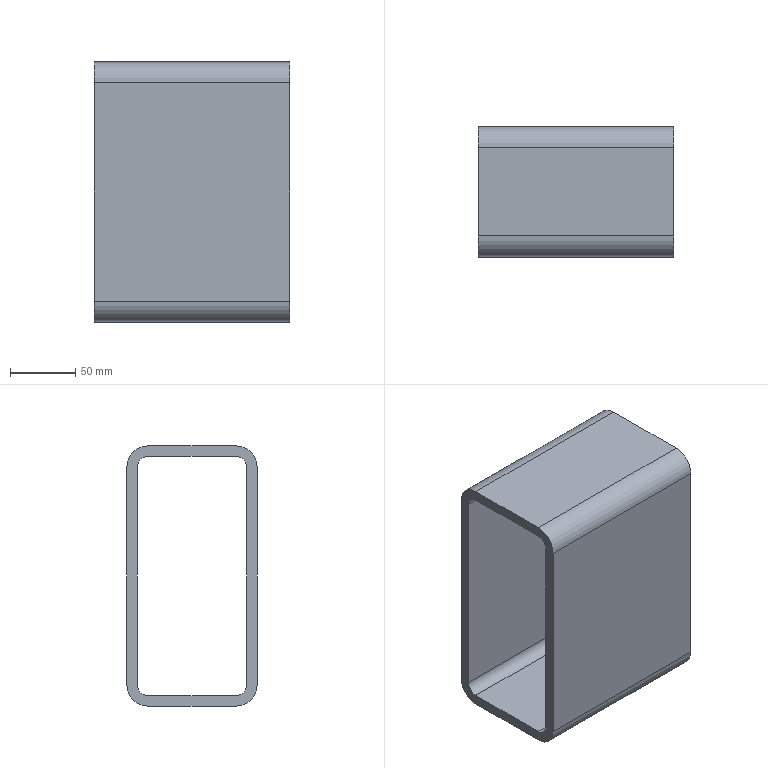Part | STEP file | 12-(flat tube 200x100x8)_default<machining> | 1 solid | 18 faces | box 150 x 100 x 200 mm | volume 656878 mm3 | plane 10 | cylinder 8 | commonest cylinder face diameters 16 x4 32 x4
STEP:
#1=CARTESIAN_POINT('',(0.,0.,0.));
#2=DIRECTION('',(0.,0.,1.));
#3=DIRECTION('',(1.,0.,0.));
#4=AXIS2_PLACEMENT_3D('',#1,#2,#3);
#5=CARTESIAN_POINT('',(0.,50.,84.));
#6=VERTEX_POINT('',#5);
#7=CARTESIAN_POINT('',(0.,34.,100.));
#8=VERTEX_POINT('',#7);
#9=CARTESIAN_POINT('',(0.,34.,84.));
#10=DIRECTION('',(1.,0.,0.));
#11=DIRECTION('',(0.,0.,-1.));
#12=AXIS2_PLACEMENT_3D('',#9,#10,#11);
#13=CIRCLE('',#12,16.);
#14=CARTESIAN_POINT('',(150.,34.,84.));
#15=DIRECTION('',(-1.,0.,0.));
#16=DIRECTION('',(0.,0.,1.));
#17=AXIS2_PLACEMENT_3D('',#14,#15,#16);
#18=CYLINDRICAL_SURFACE('',#17,16.);
#19=CARTESIAN_POINT('',(3.142,150.));
#20=DIRECTION('',(-1.,0.));
#21=VECTOR('',#20,1.);
#22=LINE('',#19,#21);
#23=(GEOMETRIC_REPRESENTATION_CONTEXT(2)PARAMETRIC_REPRESENTATION_CONTEXT()REPRESENTATION_CONTEXT('',''));
#24=DEFINITIONAL_REPRESENTATION('',(#22),#23);
#25=PCURVE('',#18,#24);
#26=CARTESIAN_POINT('',(0.,34.,84.));
#27=DIRECTION('',(1.,0.,0.));
#28=DIRECTION('',(0.,0.,-1.));
#29=AXIS2_PLACEMENT_3D('',#26,#27,#28);
#30=PLANE('',#29);
#31=CARTESIAN_POINT('',(0.,0.));
#32=DIRECTION('',(1.,0.));
#33=AXIS2_PLACEMENT_2D('',#31,#32);
#34=CIRCLE('',#33,16.);
#35=(GEOMETRIC_REPRESENTATION_CONTEXT(2)PARAMETRIC_REPRESENTATION_CONTEXT()REPRESENTATION_CONTEXT('',''));
#36=DEFINITIONAL_REPRESENTATION('',(#34),#35);
#37=PCURVE('',#30,#36);
#38=SURFACE_CURVE('',#13,(#25,#37),.PCURVE_S1.);
#39=EDGE_CURVE('',#6,#8,#38,.T.);
#40=ORIENTED_EDGE('',*,*,#39,.T.);
#41=CARTESIAN_POINT('',(150.,34.,100.));
#42=VERTEX_POINT('',#41);
#43=CARTESIAN_POINT('',(150.,34.,100.));
#44=DIRECTION('',(-1.,0.,0.));
#45=VECTOR('',#44,1.);
#46=LINE('',#43,#45);
#47=CARTESIAN_POINT('',(0.,0.));
#48=DIRECTION('',(0.,1.));
#49=VECTOR('',#48,1.);
#50=LINE('',#47,#49);
#51=(GEOMETRIC_REPRESENTATION_CONTEXT(2)PARAMETRIC_REPRESENTATION_CONTEXT()REPRESENTATION_CONTEXT('',''));
#52=DEFINITIONAL_REPRESENTATION('',(#50),#51);
#53=PCURVE('',#18,#52);
#54=CARTESIAN_POINT('',(150.,34.,100.));
#55=DIRECTION('',(0.,0.,-1.));
#56=DIRECTION('',(-1.,0.,0.));
#57=AXIS2_PLACEMENT_3D('',#54,#55,#56);
#58=PLANE('',#57);
#59=CARTESIAN_POINT('',(0.,0.));
#60=DIRECTION('',(1.,0.));
#61=VECTOR('',#60,1.);
#62=LINE('',#59,#61);
#63=(GEOMETRIC_REPRESENTATION_CONTEXT(2)PARAMETRIC_REPRESENTATION_CONTEXT()REPRESENTATION_CONTEXT('',''));
#64=DEFINITIONAL_REPRESENTATION('',(#62),#63);
#65=PCURVE('',#58,#64);
#66=SURFACE_CURVE('',#46,(#53,#65),.PCURVE_S1.);
#67=EDGE_CURVE('',#42,#8,#66,.T.);
#68=ORIENTED_EDGE('',*,*,#67,.F.);
#69=CARTESIAN_POINT('',(150.,50.,84.));
#70=VERTEX_POINT('',#69);
#71=CARTESIAN_POINT('',(150.,34.,84.));
#72=DIRECTION('',(1.,0.,0.));
#73=DIRECTION('',(0.,0.,-1.));
#74=AXIS2_PLACEMENT_3D('',#71,#72,#73);
#75=CIRCLE('',#74,16.);
#76=CARTESIAN_POINT('',(3.142,0.));
#77=DIRECTION('',(-1.,0.));
#78=VECTOR('',#77,1.);
#79=LINE('',#76,#78);
#80=(GEOMETRIC_REPRESENTATION_CONTEXT(2)PARAMETRIC_REPRESENTATION_CONTEXT()REPRESENTATION_CONTEXT('',''));
#81=DEFINITIONAL_REPRESENTATION('',(#79),#80);
#82=PCURVE('',#18,#81);
#83=CARTESIAN_POINT('',(150.,34.,84.));
#84=DIRECTION('',(1.,0.,0.));
#85=DIRECTION('',(0.,0.,-1.));
#86=AXIS2_PLACEMENT_3D('',#83,#84,#85);
#87=PLANE('',#86);
#88=CARTESIAN_POINT('',(0.,0.));
#89=DIRECTION('',(1.,0.));
#90=AXIS2_PLACEMENT_2D('',#88,#89);
#91=CIRCLE('',#90,16.);
#92=(GEOMETRIC_REPRESENTATION_CONTEXT(2)PARAMETRIC_REPRESENTATION_CONTEXT()REPRESENTATION_CONTEXT('',''));
#93=DEFINITIONAL_REPRESENTATION('',(#91),#92);
#94=PCURVE('',#87,#93);
#95=SURFACE_CURVE('',#75,(#82,#94),.PCURVE_S1.);
#96=EDGE_CURVE('',#70,#42,#95,.T.);
#97=ORIENTED_EDGE('',*,*,#96,.F.);
#98=CARTESIAN_POINT('',(150.,50.,84.));
#99=DIRECTION('',(-1.,0.,0.));
#100=VECTOR('',#99,1.);
#101=LINE('',#98,#100);
#102=CARTESIAN_POINT('',(1.571,0.));
#103=DIRECTION('',(0.,1.));
#104=VECTOR('',#103,1.);
#105=LINE('',#102,#104);
#106=(GEOMETRIC_REPRESENTATION_CONTEXT(2)PARAMETRIC_REPRESENTATION_CONTEXT()REPRESENTATION_CONTEXT('',''));
#107=DEFINITIONAL_REPRESENTATION('',(#105),#106);
#108=PCURVE('',#18,#107);
#109=CARTESIAN_POINT('',(150.,50.,84.));
#110=DIRECTION('',(0.,-1.,0.));
#111=DIRECTION('',(0.,0.,-1.));
#112=AXIS2_PLACEMENT_3D('',#109,#110,#111);
#113=PLANE('',#112);
#114=CARTESIAN_POINT('',(0.,0.));
#115=DIRECTION('',(0.,-1.));
#116=VECTOR('',#115,1.);
#117=LINE('',#114,#116);
#118=(GEOMETRIC_REPRESENTATION_CONTEXT(2)PARAMETRIC_REPRESENTATION_CONTEXT()REPRESENTATION_CONTEXT('',''));
#119=DEFINITIONAL_REPRESENTATION('',(#117),#118);
#120=PCURVE('',#113,#119);
#121=SURFACE_CURVE('',#101,(#108,#120),.PCURVE_S1.);
#122=EDGE_CURVE('',#70,#6,#121,.T.);
#123=ORIENTED_EDGE('',*,*,#122,.T.);
#124=EDGE_LOOP('',(#40,#68,#97,#123));
#125=FACE_BOUND('',#124,.T.);
#126=ADVANCED_FACE('',(#125),#18,.T.);
#127=CARTESIAN_POINT('',(0.,-34.,100.));
#128=VERTEX_POINT('',#127);
#129=CARTESIAN_POINT('',(0.,34.,100.));
#130=DIRECTION('',(0.,-1.,0.));
#131=VECTOR('',#130,1.);
#132=LINE('',#129,#131);
#133=CARTESIAN_POINT('',(150.,0.));
#134=DIRECTION('',(0.,-1.));
#135=VECTOR('',#134,1.);
#136=LINE('',#133,#135);
#137=(GEOMETRIC_REPRESENTATION_CONTEXT(2)PARAMETRIC_REPRESENTATION_CONTEXT()REPRESENTATION_CONTEXT('',''));
#138=DEFINITIONAL_REPRESENTATION('',(#136),#137);
#139=PCURVE('',#58,#138);
#140=CARTESIAN_POINT('',(-16.,0.));
#141=DIRECTION('',(0.,-1.));
#142=VECTOR('',#141,1.);
#143=LINE('',#140,#142);
#144=(GEOMETRIC_REPRESENTATION_CONTEXT(2)PARAMETRIC_REPRESENTATION_CONTEXT()REPRESENTATION_CONTEXT('',''));
#145=DEFINITIONAL_REPRESENTATION('',(#143),#144);
#146=PCURVE('',#30,#145);
#147=SURFACE_CURVE('',#132,(#139,#146),.PCURVE_S1.);
#148=EDGE_CURVE('',#8,#128,#147,.T.);
#149=ORIENTED_EDGE('',*,*,#148,.T.);
#150=CARTESIAN_POINT('',(150.,-34.,100.));
#151=VERTEX_POINT('',#150);
#152=CARTESIAN_POINT('',(150.,-34.,100.));
#153=DIRECTION('',(-1.,0.,0.));
#154=VECTOR('',#153,1.);
#155=LINE('',#152,#154);
#156=CARTESIAN_POINT('',(0.,-68.));
#157=DIRECTION('',(1.,0.));
#158=VECTOR('',#157,1.);
#159=LINE('',#156,#158);
#160=(GEOMETRIC_REPRESENTATION_CONTEXT(2)PARAMETRIC_REPRESENTATION_CONTEXT()REPRESENTATION_CONTEXT('',''));
#161=DEFINITIONAL_REPRESENTATION('',(#159),#160);
#162=PCURVE('',#58,#161);
#163=CARTESIAN_POINT('',(150.,-34.,84.));
#164=DIRECTION('',(-1.,0.,0.));
#165=DIRECTION('',(0.,0.,1.));
#166=AXIS2_PLACEMENT_3D('',#163,#164,#165);
#167=CYLINDRICAL_SURFACE('',#166,16.);
#168=CARTESIAN_POINT('',(6.283,0.));
#169=DIRECTION('',(0.,1.));
#170=VECTOR('',#169,1.);
#171=LINE('',#168,#170);
#172=(GEOMETRIC_REPRESENTATION_CONTEXT(2)PARAMETRIC_REPRESENTATION_CONTEXT()REPRESENTATION_CONTEXT('',''));
#173=DEFINITIONAL_REPRESENTATION('',(#171),#172);
#174=PCURVE('',#167,#173);
#175=SURFACE_CURVE('',#155,(#162,#174),.PCURVE_S1.);
#176=EDGE_CURVE('',#151,#128,#175,.T.);
#177=ORIENTED_EDGE('',*,*,#176,.F.);
#178=CARTESIAN_POINT('',(150.,34.,100.));
#179=DIRECTION('',(0.,-1.,0.));
#180=VECTOR('',#179,1.);
#181=LINE('',#178,#180);
#182=CARTESIAN_POINT('',(0.,0.));
#183=DIRECTION('',(0.,-1.));
#184=VECTOR('',#183,1.);
#185=LINE('',#182,#184);
#186=(GEOMETRIC_REPRESENTATION_CONTEXT(2)PARAMETRIC_REPRESENTATION_CONTEXT()REPRESENTATION_CONTEXT('',''));
#187=DEFINITIONAL_REPRESENTATION('',(#185),#186);
#188=PCURVE('',#58,#187);
#189=CARTESIAN_POINT('',(-16.,0.));
#190=DIRECTION('',(0.,-1.));
#191=VECTOR('',#190,1.);
#192=LINE('',#189,#191);
#193=(GEOMETRIC_REPRESENTATION_CONTEXT(2)PARAMETRIC_REPRESENTATION_CONTEXT()REPRESENTATION_CONTEXT('',''));
#194=DEFINITIONAL_REPRESENTATION('',(#192),#193);
#195=PCURVE('',#87,#194);
#196=SURFACE_CURVE('',#181,(#188,#195),.PCURVE_S1.);
#197=EDGE_CURVE('',#42,#151,#196,.T.);
#198=ORIENTED_EDGE('',*,*,#197,.F.);
#199=ORIENTED_EDGE('',*,*,#67,.T.);
#200=EDGE_LOOP('',(#149,#177,#198,#199));
#201=FACE_BOUND('',#200,.T.);
#202=ADVANCED_FACE('',(#201),#58,.F.);
#203=CARTESIAN_POINT('',(0.,-50.,84.));
#204=VERTEX_POINT('',#203);
#205=CARTESIAN_POINT('',(0.,-34.,84.));
#206=DIRECTION('',(1.,0.,0.));
#207=DIRECTION('',(0.,0.,-1.));
#208=AXIS2_PLACEMENT_3D('',#205,#206,#207);
#209=CIRCLE('',#208,16.);
#210=CARTESIAN_POINT('',(9.425,150.));
#211=DIRECTION('',(-1.,0.));
#212=VECTOR('',#211,1.);
#213=LINE('',#210,#212);
#214=(GEOMETRIC_REPRESENTATION_CONTEXT(2)PARAMETRIC_REPRESENTATION_CONTEXT()REPRESENTATION_CONTEXT('',''));
#215=DEFINITIONAL_REPRESENTATION('',(#213),#214);
#216=PCURVE('',#167,#215);
#217=CARTESIAN_POINT('',(0.,-68.));
#218=DIRECTION('',(1.,0.));
#219=AXIS2_PLACEMENT_2D('',#217,#218);
#220=CIRCLE('',#219,16.);
#221=(GEOMETRIC_REPRESENTATION_CONTEXT(2)PARAMETRIC_REPRESENTATION_CONTEXT()REPRESENTATION_CONTEXT('',''));
#222=DEFINITIONAL_REPRESENTATION('',(#220),#221);
#223=PCURVE('',#30,#222);
#224=SURFACE_CURVE('',#209,(#216,#223),.PCURVE_S1.);
#225=EDGE_CURVE('',#128,#204,#224,.T.);
#226=ORIENTED_EDGE('',*,*,#225,.T.);
#227=CARTESIAN_POINT('',(150.,-50.,84.));
#228=VERTEX_POINT('',#227);
#229=CARTESIAN_POINT('',(150.,-50.,84.));
#230=DIRECTION('',(-1.,0.,0.));
#231=VECTOR('',#230,1.);
#232=LINE('',#229,#231);
#233=CARTESIAN_POINT('',(4.712,0.));
#234=DIRECTION('',(0.,1.));
#235=VECTOR('',#234,1.);
#236=LINE('',#233,#235);
#237=(GEOMETRIC_REPRESENTATION_CONTEXT(2)PARAMETRIC_REPRESENTATION_CONTEXT()REPRESENTATION_CONTEXT('',''));
#238=DEFINITIONAL_REPRESENTATION('',(#236),#237);
#239=PCURVE('',#167,#238);
#240=CARTESIAN_POINT('',(150.,-50.,-84.));
#241=DIRECTION('',(0.,1.,0.));
#242=DIRECTION('',(0.,0.,1.));
#243=AXIS2_PLACEMENT_3D('',#240,#241,#242);
#244=PLANE('',#243);
#245=CARTESIAN_POINT('',(168.,0.));
#246=DIRECTION('',(0.,-1.));
#247=VECTOR('',#246,1.);
#248=LINE('',#245,#247);
#249=(GEOMETRIC_REPRESENTATION_CONTEXT(2)PARAMETRIC_REPRESENTATION_CONTEXT()REPRESENTATION_CONTEXT('',''));
#250=DEFINITIONAL_REPRESENTATION('',(#248),#249);
#251=PCURVE('',#244,#250);
#252=SURFACE_CURVE('',#232,(#239,#251),.PCURVE_S1.);
#253=EDGE_CURVE('',#228,#204,#252,.T.);
#254=ORIENTED_EDGE('',*,*,#253,.F.);
#255=CARTESIAN_POINT('',(150.,-34.,84.));
#256=DIRECTION('',(1.,0.,0.));
#257=DIRECTION('',(0.,0.,-1.));
#258=AXIS2_PLACEMENT_3D('',#255,#256,#257);
#259=CIRCLE('',#258,16.);
#260=CARTESIAN_POINT('',(9.425,0.));
#261=DIRECTION('',(-1.,0.));
#262=VECTOR('',#261,1.);
#263=LINE('',#260,#262);
#264=(GEOMETRIC_REPRESENTATION_CONTEXT(2)PARAMETRIC_REPRESENTATION_CONTEXT()REPRESENTATION_CONTEXT('',''));
#265=DEFINITIONAL_REPRESENTATION('',(#263),#264);
#266=PCURVE('',#167,#265);
#267=CARTESIAN_POINT('',(0.,-68.));
#268=DIRECTION('',(1.,0.));
#269=AXIS2_PLACEMENT_2D('',#267,#268);
#270=CIRCLE('',#269,16.);
#271=(GEOMETRIC_REPRESENTATION_CONTEXT(2)PARAMETRIC_REPRESENTATION_CONTEXT()REPRESENTATION_CONTEXT('',''));
#272=DEFINITIONAL_REPRESENTATION('',(#270),#271);
#273=PCURVE('',#87,#272);
#274=SURFACE_CURVE('',#259,(#266,#273),.PCURVE_S1.);
#275=EDGE_CURVE('',#151,#228,#274,.T.);
#276=ORIENTED_EDGE('',*,*,#275,.F.);
#277=ORIENTED_EDGE('',*,*,#176,.T.);
#278=EDGE_LOOP('',(#226,#254,#276,#277));
#279=FACE_BOUND('',#278,.T.);
#280=ADVANCED_FACE('',(#279),#167,.T.);
#281=CARTESIAN_POINT('',(0.,-50.,-84.));
#282=VERTEX_POINT('',#281);
#283=CARTESIAN_POINT('',(0.,-50.,-84.));
#284=DIRECTION('',(0.,0.,-1.));
#285=VECTOR('',#284,1.);
#286=LINE('',#283,#285);
#287=CARTESIAN_POINT('',(0.,-150.));
#288=DIRECTION('',(-1.,0.));
#289=VECTOR('',#288,1.);
#290=LINE('',#287,#289);
#291=(GEOMETRIC_REPRESENTATION_CONTEXT(2)PARAMETRIC_REPRESENTATION_CONTEXT()REPRESENTATION_CONTEXT('',''));
#292=DEFINITIONAL_REPRESENTATION('',(#290),#291);
#293=PCURVE('',#244,#292);
#294=CARTESIAN_POINT('',(168.,-84.));
#295=DIRECTION('',(1.,0.));
#296=VECTOR('',#295,1.);
#297=LINE('',#294,#296);
#298=(GEOMETRIC_REPRESENTATION_CONTEXT(2)PARAMETRIC_REPRESENTATION_CONTEXT()REPRESENTATION_CONTEXT('',''));
#299=DEFINITIONAL_REPRESENTATION('',(#297),#298);
#300=PCURVE('',#30,#299);
#301=SURFACE_CURVE('',#286,(#293,#300),.PCURVE_S1.);
#302=EDGE_CURVE('',#204,#282,#301,.T.);
#303=ORIENTED_EDGE('',*,*,#302,.T.);
#304=CARTESIAN_POINT('',(150.,-50.,-84.));
#305=VERTEX_POINT('',#304);
#306=CARTESIAN_POINT('',(150.,-50.,-84.));
#307=DIRECTION('',(-1.,0.,0.));
#308=VECTOR('',#307,1.);
#309=LINE('',#306,#308);
#310=CARTESIAN_POINT('',(0.,0.));
#311=DIRECTION('',(0.,-1.));
#312=VECTOR('',#311,1.);
#313=LINE('',#310,#312);
#314=(GEOMETRIC_REPRESENTATION_CONTEXT(2)PARAMETRIC_REPRESENTATION_CONTEXT()REPRESENTATION_CONTEXT('',''));
#315=DEFINITIONAL_REPRESENTATION('',(#313),#314);
#316=PCURVE('',#244,#315);
#317=CARTESIAN_POINT('',(150.,-34.,-84.));
#318=DIRECTION('',(-1.,0.,0.));
#319=DIRECTION('',(0.,0.,1.));
#320=AXIS2_PLACEMENT_3D('',#317,#318,#319);
#321=CYLINDRICAL_SURFACE('',#320,16.);
#322=CARTESIAN_POINT('',(4.712,0.));
#323=DIRECTION('',(0.,1.));
#324=VECTOR('',#323,1.);
#325=LINE('',#322,#324);
#326=(GEOMETRIC_REPRESENTATION_CONTEXT(2)PARAMETRIC_REPRESENTATION_CONTEXT()REPRESENTATION_CONTEXT('',''));
#327=DEFINITIONAL_REPRESENTATION('',(#325),#326);
#328=PCURVE('',#321,#327);
#329=SURFACE_CURVE('',#309,(#316,#328),.PCURVE_S1.);
#330=EDGE_CURVE('',#305,#282,#329,.T.);
#331=ORIENTED_EDGE('',*,*,#330,.F.);
#332=CARTESIAN_POINT('',(150.,-50.,-84.));
#333=DIRECTION('',(0.,0.,-1.));
#334=VECTOR('',#333,1.);
#335=LINE('',#332,#334);
#336=CARTESIAN_POINT('',(0.,0.));
#337=DIRECTION('',(-1.,0.));
#338=VECTOR('',#337,1.);
#339=LINE('',#336,#338);
#340=(GEOMETRIC_REPRESENTATION_CONTEXT(2)PARAMETRIC_REPRESENTATION_CONTEXT()REPRESENTATION_CONTEXT('',''));
#341=DEFINITIONAL_REPRESENTATION('',(#339),#340);
#342=PCURVE('',#244,#341);
#343=CARTESIAN_POINT('',(168.,-84.));
#344=DIRECTION('',(1.,0.));
#345=VECTOR('',#344,1.);
#346=LINE('',#343,#345);
#347=(GEOMETRIC_REPRESENTATION_CONTEXT(2)PARAMETRIC_REPRESENTATION_CONTEXT()REPRESENTATION_CONTEXT('',''));
#348=DEFINITIONAL_REPRESENTATION('',(#346),#347);
#349=PCURVE('',#87,#348);
#350=SURFACE_CURVE('',#335,(#342,#349),.PCURVE_S1.);
#351=EDGE_CURVE('',#228,#305,#350,.T.);
#352=ORIENTED_EDGE('',*,*,#351,.F.);
#353=ORIENTED_EDGE('',*,*,#253,.T.);
#354=EDGE_LOOP('',(#303,#331,#352,#353));
#355=FACE_BOUND('',#354,.T.);
#356=ADVANCED_FACE('',(#355),#244,.F.);
#357=CARTESIAN_POINT('',(0.,-34.,-100.));
#358=VERTEX_POINT('',#357);
#359=CARTESIAN_POINT('',(0.,-34.,-84.));
#360=DIRECTION('',(1.,0.,0.));
#361=DIRECTION('',(0.,0.,-1.));
#362=AXIS2_PLACEMENT_3D('',#359,#360,#361);
#363=CIRCLE('',#362,16.);
#364=CARTESIAN_POINT('',(9.425,150.));
#365=DIRECTION('',(-1.,0.));
#366=VECTOR('',#365,1.);
#367=LINE('',#364,#366);
#368=(GEOMETRIC_REPRESENTATION_CONTEXT(2)PARAMETRIC_REPRESENTATION_CONTEXT()REPRESENTATION_CONTEXT('',''));
#369=DEFINITIONAL_REPRESENTATION('',(#367),#368);
#370=PCURVE('',#321,#369);
#371=CARTESIAN_POINT('',(168.,-68.));
#372=DIRECTION('',(1.,0.));
#373=AXIS2_PLACEMENT_2D('',#371,#372);
#374=CIRCLE('',#373,16.);
#375=(GEOMETRIC_REPRESENTATION_CONTEXT(2)PARAMETRIC_REPRESENTATION_CONTEXT()REPRESENTATION_CONTEXT('',''));
#376=DEFINITIONAL_REPRESENTATION('',(#374),#375);
#377=PCURVE('',#30,#376);
#378=SURFACE_CURVE('',#363,(#370,#377),.PCURVE_S1.);
#379=EDGE_CURVE('',#282,#358,#378,.T.);
#380=ORIENTED_EDGE('',*,*,#379,.T.);
#381=CARTESIAN_POINT('',(150.,-34.,-100.));
#382=VERTEX_POINT('',#381);
#383=CARTESIAN_POINT('',(150.,-34.,-100.));
#384=DIRECTION('',(-1.,0.,0.));
#385=VECTOR('',#384,1.);
#386=LINE('',#383,#385);
#387=CARTESIAN_POINT('',(3.142,0.));
#388=DIRECTION('',(0.,1.));
#389=VECTOR('',#388,1.);
#390=LINE('',#387,#389);
#391=(GEOMETRIC_REPRESENTATION_CONTEXT(2)PARAMETRIC_REPRESENTATION_CONTEXT()REPRESENTATION_CONTEXT('',''));
#392=DEFINITIONAL_REPRESENTATION('',(#390),#391);
#393=PCURVE('',#321,#392);
#394=CARTESIAN_POINT('',(150.,-34.,-100.));
#395=DIRECTION('',(0.,0.,1.));
#396=DIRECTION('',(1.,0.,0.));
#397=AXIS2_PLACEMENT_3D('',#394,#395,#396);
#398=PLANE('',#397);
#399=CARTESIAN_POINT('',(0.,0.));
#400=DIRECTION('',(-1.,0.));
#401=VECTOR('',#400,1.);
#402=LINE('',#399,#401);
#403=(GEOMETRIC_REPRESENTATION_CONTEXT(2)PARAMETRIC_REPRESENTATION_CONTEXT()REPRESENTATION_CONTEXT('',''));
#404=DEFINITIONAL_REPRESENTATION('',(#402),#403);
#405=PCURVE('',#398,#404);
#406=SURFACE_CURVE('',#386,(#393,#405),.PCURVE_S1.);
#407=EDGE_CURVE('',#382,#358,#406,.T.);
#408=ORIENTED_EDGE('',*,*,#407,.F.);
#409=CARTESIAN_POINT('',(150.,-34.,-84.));
#410=DIRECTION('',(1.,0.,0.));
#411=DIRECTION('',(0.,0.,-1.));
#412=AXIS2_PLACEMENT_3D('',#409,#410,#411);
#413=CIRCLE('',#412,16.);
#414=CARTESIAN_POINT('',(9.425,0.));
#415=DIRECTION('',(-1.,0.));
#416=VECTOR('',#415,1.);
#417=LINE('',#414,#416);
#418=(GEOMETRIC_REPRESENTATION_CONTEXT(2)PARAMETRIC_REPRESENTATION_CONTEXT()REPRESENTATION_CONTEXT('',''));
#419=DEFINITIONAL_REPRESENTATION('',(#417),#418);
#420=PCURVE('',#321,#419);
#421=CARTESIAN_POINT('',(168.,-68.));
#422=DIRECTION('',(1.,0.));
#423=AXIS2_PLACEMENT_2D('',#421,#422);
#424=CIRCLE('',#423,16.);
#425=(GEOMETRIC_REPRESENTATION_CONTEXT(2)PARAMETRIC_REPRESENTATION_CONTEXT()REPRESENTATION_CONTEXT('',''));
#426=DEFINITIONAL_REPRESENTATION('',(#424),#425);
#427=PCURVE('',#87,#426);
#428=SURFACE_CURVE('',#413,(#420,#427),.PCURVE_S1.);
#429=EDGE_CURVE('',#305,#382,#428,.T.);
#430=ORIENTED_EDGE('',*,*,#429,.F.);
#431=ORIENTED_EDGE('',*,*,#330,.T.);
#432=EDGE_LOOP('',(#380,#408,#430,#431));
#433=FACE_BOUND('',#432,.T.);
#434=ADVANCED_FACE('',(#433),#321,.T.);
#435=CARTESIAN_POINT('',(0.,34.,-100.));
#436=VERTEX_POINT('',#435);
#437=CARTESIAN_POINT('',(0.,-34.,-100.));
#438=DIRECTION('',(0.,1.,0.));
#439=VECTOR('',#438,1.);
#440=LINE('',#437,#439);
#441=CARTESIAN_POINT('',(-150.,0.));
#442=DIRECTION('',(0.,1.));
#443=VECTOR('',#442,1.);
#444=LINE('',#441,#443);
#445=(GEOMETRIC_REPRESENTATION_CONTEXT(2)PARAMETRIC_REPRESENTATION_CONTEXT()REPRESENTATION_CONTEXT('',''));
#446=DEFINITIONAL_REPRESENTATION('',(#444),#445);
#447=PCURVE('',#398,#446);
#448=CARTESIAN_POINT('',(184.,-68.));
#449=DIRECTION('',(0.,1.));
#450=VECTOR('',#449,1.);
#451=LINE('',#448,#450);
#452=(GEOMETRIC_REPRESENTATION_CONTEXT(2)PARAMETRIC_REPRESENTATION_CONTEXT()REPRESENTATION_CONTEXT('',''));
#453=DEFINITIONAL_REPRESENTATION('',(#451),#452);
#454=PCURVE('',#30,#453);
#455=SURFACE_CURVE('',#440,(#447,#454),.PCURVE_S1.);
#456=EDGE_CURVE('',#358,#436,#455,.T.);
#457=ORIENTED_EDGE('',*,*,#456,.T.);
#458=CARTESIAN_POINT('',(150.,34.,-100.));
#459=VERTEX_POINT('',#458);
#460=CARTESIAN_POINT('',(150.,34.,-100.));
#461=DIRECTION('',(-1.,0.,0.));
#462=VECTOR('',#461,1.);
#463=LINE('',#460,#462);
#464=CARTESIAN_POINT('',(0.,68.));
#465=DIRECTION('',(-1.,0.));
#466=VECTOR('',#465,1.);
#467=LINE('',#464,#466);
#468=(GEOMETRIC_REPRESENTATION_CONTEXT(2)PARAMETRIC_REPRESENTATION_CONTEXT()REPRESENTATION_CONTEXT('',''));
#469=DEFINITIONAL_REPRESENTATION('',(#467),#468);
#470=PCURVE('',#398,#469);
#471=CARTESIAN_POINT('',(150.,34.,-84.));
#472=DIRECTION('',(-1.,0.,0.));
#473=DIRECTION('',(0.,0.,1.));
#474=AXIS2_PLACEMENT_3D('',#471,#472,#473);
#475=CYLINDRICAL_SURFACE('',#474,16.);
#476=CARTESIAN_POINT('',(3.142,0.));
#477=DIRECTION('',(0.,1.));
#478=VECTOR('',#477,1.);
#479=LINE('',#476,#478);
#480=(GEOMETRIC_REPRESENTATION_CONTEXT(2)PARAMETRIC_REPRESENTATION_CONTEXT()REPRESENTATION_CONTEXT('',''));
#481=DEFINITIONAL_REPRESENTATION('',(#479),#480);
#482=PCURVE('',#475,#481);
#483=SURFACE_CURVE('',#463,(#470,#482),.PCURVE_S1.);
#484=EDGE_CURVE('',#459,#436,#483,.T.);
#485=ORIENTED_EDGE('',*,*,#484,.F.);
#486=CARTESIAN_POINT('',(150.,-34.,-100.));
#487=DIRECTION('',(0.,1.,0.));
#488=VECTOR('',#487,1.);
#489=LINE('',#486,#488);
#490=CARTESIAN_POINT('',(0.,0.));
#491=DIRECTION('',(0.,1.));
#492=VECTOR('',#491,1.);
#493=LINE('',#490,#492);
#494=(GEOMETRIC_REPRESENTATION_CONTEXT(2)PARAMETRIC_REPRESENTATION_CONTEXT()REPRESENTATION_CONTEXT('',''));
#495=DEFINITIONAL_REPRESENTATION('',(#493),#494);
#496=PCURVE('',#398,#495);
#497=CARTESIAN_POINT('',(184.,-68.));
#498=DIRECTION('',(0.,1.));
#499=VECTOR('',#498,1.);
#500=LINE('',#497,#499);
#501=(GEOMETRIC_REPRESENTATION_CONTEXT(2)PARAMETRIC_REPRESENTATION_CONTEXT()REPRESENTATION_CONTEXT('',''));
#502=DEFINITIONAL_REPRESENTATION('',(#500),#501);
#503=PCURVE('',#87,#502);
#504=SURFACE_CURVE('',#489,(#496,#503),.PCURVE_S1.);
#505=EDGE_CURVE('',#382,#459,#504,.T.);
#506=ORIENTED_EDGE('',*,*,#505,.F.);
#507=ORIENTED_EDGE('',*,*,#407,.T.);
#508=EDGE_LOOP('',(#457,#485,#506,#507));
#509=FACE_BOUND('',#508,.T.);
#510=ADVANCED_FACE('',(#509),#398,.F.);
#511=CARTESIAN_POINT('',(0.,50.,-84.));
#512=VERTEX_POINT('',#511);
#513=CARTESIAN_POINT('',(0.,34.,-84.));
#514=DIRECTION('',(1.,0.,0.));
#515=DIRECTION('',(0.,0.,-1.));
#516=AXIS2_PLACEMENT_3D('',#513,#514,#515);
#517=CIRCLE('',#516,16.);
#518=CARTESIAN_POINT('',(3.142,150.));
#519=DIRECTION('',(-1.,0.));
#520=VECTOR('',#519,1.);
#521=LINE('',#518,#520);
#522=(GEOMETRIC_REPRESENTATION_CONTEXT(2)PARAMETRIC_REPRESENTATION_CONTEXT()REPRESENTATION_CONTEXT('',''));
#523=DEFINITIONAL_REPRESENTATION('',(#521),#522);
#524=PCURVE('',#475,#523);
#525=CARTESIAN_POINT('',(168.,0.));
#526=DIRECTION('',(1.,0.));
#527=AXIS2_PLACEMENT_2D('',#525,#526);
#528=CIRCLE('',#527,16.);
#529=(GEOMETRIC_REPRESENTATION_CONTEXT(2)PARAMETRIC_REPRESENTATION_CONTEXT()REPRESENTATION_CONTEXT('',''));
#530=DEFINITIONAL_REPRESENTATION('',(#528),#529);
#531=PCURVE('',#30,#530);
#532=SURFACE_CURVE('',#517,(#524,#531),.PCURVE_S1.);
#533=EDGE_CURVE('',#436,#512,#532,.T.);
#534=ORIENTED_EDGE('',*,*,#533,.T.);
#535=CARTESIAN_POINT('',(150.,50.,-84.));
#536=VERTEX_POINT('',#535);
#537=CARTESIAN_POINT('',(150.,50.,-84.));
#538=DIRECTION('',(-1.,0.,0.));
#539=VECTOR('',#538,1.);
#540=LINE('',#537,#539);
#541=CARTESIAN_POINT('',(1.571,0.));
#542=DIRECTION('',(0.,1.));
#543=VECTOR('',#542,1.);
#544=LINE('',#541,#543);
#545=(GEOMETRIC_REPRESENTATION_CONTEXT(2)PARAMETRIC_REPRESENTATION_CONTEXT()REPRESENTATION_CONTEXT('',''));
#546=DEFINITIONAL_REPRESENTATION('',(#544),#545);
#547=PCURVE('',#475,#546);
#548=CARTESIAN_POINT('',(168.,0.));
#549=DIRECTION('',(0.,-1.));
#550=VECTOR('',#549,1.);
#551=LINE('',#548,#550);
#552=(GEOMETRIC_REPRESENTATION_CONTEXT(2)PARAMETRIC_REPRESENTATION_CONTEXT()REPRESENTATION_CONTEXT('',''));
#553=DEFINITIONAL_REPRESENTATION('',(#551),#552);
#554=PCURVE('',#113,#553);
#555=SURFACE_CURVE('',#540,(#547,#554),.PCURVE_S1.);
#556=EDGE_CURVE('',#536,#512,#555,.T.);
#557=ORIENTED_EDGE('',*,*,#556,.F.);
#558=CARTESIAN_POINT('',(150.,34.,-84.));
#559=DIRECTION('',(1.,0.,0.));
#560=DIRECTION('',(0.,0.,-1.));
#561=AXIS2_PLACEMENT_3D('',#558,#559,#560);
#562=CIRCLE('',#561,16.);
#563=CARTESIAN_POINT('',(3.142,0.));
#564=DIRECTION('',(-1.,0.));
#565=VECTOR('',#564,1.);
#566=LINE('',#563,#565);
#567=(GEOMETRIC_REPRESENTATION_CONTEXT(2)PARAMETRIC_REPRESENTATION_CONTEXT()REPRESENTATION_CONTEXT('',''));
#568=DEFINITIONAL_REPRESENTATION('',(#566),#567);
#569=PCURVE('',#475,#568);
#570=CARTESIAN_POINT('',(168.,0.));
#571=DIRECTION('',(1.,0.));
#572=AXIS2_PLACEMENT_2D('',#570,#571);
#573=CIRCLE('',#572,16.);
#574=(GEOMETRIC_REPRESENTATION_CONTEXT(2)PARAMETRIC_REPRESENTATION_CONTEXT()REPRESENTATION_CONTEXT('',''));
#575=DEFINITIONAL_REPRESENTATION('',(#573),#574);
#576=PCURVE('',#87,#575);
#577=SURFACE_CURVE('',#562,(#569,#576),.PCURVE_S1.);
#578=EDGE_CURVE('',#459,#536,#577,.T.);
#579=ORIENTED_EDGE('',*,*,#578,.F.);
#580=ORIENTED_EDGE('',*,*,#484,.T.);
#581=EDGE_LOOP('',(#534,#557,#579,#580));
#582=FACE_BOUND('',#581,.T.);
#583=ADVANCED_FACE('',(#582),#475,.T.);
#584=CARTESIAN_POINT('',(150.,-42.,84.));
#585=VERTEX_POINT('',#584);
#586=CARTESIAN_POINT('',(0.,-42.,84.));
#587=VERTEX_POINT('',#586);
#588=CARTESIAN_POINT('',(150.,-42.,84.));
#589=DIRECTION('',(-1.,0.,0.));
#590=VECTOR('',#589,1.);
#591=LINE('',#588,#590);
#592=CARTESIAN_POINT('',(150.,-34.,84.));
#593=DIRECTION('',(-1.,0.,0.));
#594=DIRECTION('',(0.,0.,1.));
#595=AXIS2_PLACEMENT_3D('',#592,#593,#594);
#596=CYLINDRICAL_SURFACE('',#595,8.);
#597=CARTESIAN_POINT('',(4.712,0.));
#598=DIRECTION('',(0.,1.));
#599=VECTOR('',#598,1.);
#600=LINE('',#597,#599);
#601=(GEOMETRIC_REPRESENTATION_CONTEXT(2)PARAMETRIC_REPRESENTATION_CONTEXT()REPRESENTATION_CONTEXT('',''));
#602=DEFINITIONAL_REPRESENTATION('',(#600),#601);
#603=PCURVE('',#596,#602);
#604=CARTESIAN_POINT('',(150.,-42.,-84.));
#605=DIRECTION('',(0.,1.,0.));
#606=DIRECTION('',(0.,0.,1.));
#607=AXIS2_PLACEMENT_3D('',#604,#605,#606);
#608=PLANE('',#607);
#609=CARTESIAN_POINT('',(168.,0.));
#610=DIRECTION('',(0.,-1.));
#611=VECTOR('',#610,1.);
#612=LINE('',#609,#611);
#613=(GEOMETRIC_REPRESENTATION_CONTEXT(2)PARAMETRIC_REPRESENTATION_CONTEXT()REPRESENTATION_CONTEXT('',''));
#614=DEFINITIONAL_REPRESENTATION('',(#612),#613);
#615=PCURVE('',#608,#614);
#616=SURFACE_CURVE('',#591,(#603,#615),.PCURVE_S1.);
#617=EDGE_CURVE('',#585,#587,#616,.T.);
#618=ORIENTED_EDGE('',*,*,#617,.F.);
#619=CARTESIAN_POINT('',(150.,-34.,92.));
#620=VERTEX_POINT('',#619);
#621=CARTESIAN_POINT('',(150.,-34.,84.));
#622=DIRECTION('',(1.,0.,0.));
#623=DIRECTION('',(0.,0.,-1.));
#624=AXIS2_PLACEMENT_3D('',#621,#622,#623);
#625=CIRCLE('',#624,8.);
#626=CARTESIAN_POINT('',(9.425,0.));
#627=DIRECTION('',(-1.,0.));
#628=VECTOR('',#627,1.);
#629=LINE('',#626,#628);
#630=(GEOMETRIC_REPRESENTATION_CONTEXT(2)PARAMETRIC_REPRESENTATION_CONTEXT()REPRESENTATION_CONTEXT('',''));
#631=DEFINITIONAL_REPRESENTATION('',(#629),#630);
#632=PCURVE('',#596,#631);
#633=CARTESIAN_POINT('',(0.,-68.));
#634=DIRECTION('',(1.,0.));
#635=AXIS2_PLACEMENT_2D('',#633,#634);
#636=CIRCLE('',#635,8.);
#637=(GEOMETRIC_REPRESENTATION_CONTEXT(2)PARAMETRIC_REPRESENTATION_CONTEXT()REPRESENTATION_CONTEXT('',''));
#638=DEFINITIONAL_REPRESENTATION('',(#636),#637);
#639=PCURVE('',#87,#638);
#640=SURFACE_CURVE('',#625,(#632,#639),.PCURVE_S1.);
#641=EDGE_CURVE('',#620,#585,#640,.T.);
#642=ORIENTED_EDGE('',*,*,#641,.F.);
#643=CARTESIAN_POINT('',(0.,-34.,92.));
#644=VERTEX_POINT('',#643);
#645=CARTESIAN_POINT('',(150.,-34.,92.));
#646=DIRECTION('',(-1.,0.,0.));
#647=VECTOR('',#646,1.);
#648=LINE('',#645,#647);
#649=CARTESIAN_POINT('',(6.283,0.));
#650=DIRECTION('',(0.,1.));
#651=VECTOR('',#650,1.);
#652=LINE('',#649,#651);
#653=(GEOMETRIC_REPRESENTATION_CONTEXT(2)PARAMETRIC_REPRESENTATION_CONTEXT()REPRESENTATION_CONTEXT('',''));
#654=DEFINITIONAL_REPRESENTATION('',(#652),#653);
#655=PCURVE('',#596,#654);
#656=CARTESIAN_POINT('',(150.,34.,92.));
#657=DIRECTION('',(0.,0.,-1.));
#658=DIRECTION('',(-1.,0.,0.));
#659=AXIS2_PLACEMENT_3D('',#656,#657,#658);
#660=PLANE('',#659);
#661=CARTESIAN_POINT('',(0.,-68.));
#662=DIRECTION('',(1.,0.));
#663=VECTOR('',#662,1.);
#664=LINE('',#661,#663);
#665=(GEOMETRIC_REPRESENTATION_CONTEXT(2)PARAMETRIC_REPRESENTATION_CONTEXT()REPRESENTATION_CONTEXT('',''));
#666=DEFINITIONAL_REPRESENTATION('',(#664),#665);
#667=PCURVE('',#660,#666);
#668=SURFACE_CURVE('',#648,(#655,#667),.PCURVE_S1.);
#669=EDGE_CURVE('',#620,#644,#668,.T.);
#670=ORIENTED_EDGE('',*,*,#669,.T.);
#671=CARTESIAN_POINT('',(0.,-34.,84.));
#672=DIRECTION('',(1.,0.,0.));
#673=DIRECTION('',(0.,0.,-1.));
#674=AXIS2_PLACEMENT_3D('',#671,#672,#673);
#675=CIRCLE('',#674,8.);
#676=CARTESIAN_POINT('',(9.425,150.));
#677=DIRECTION('',(-1.,0.));
#678=VECTOR('',#677,1.);
#679=LINE('',#676,#678);
#680=(GEOMETRIC_REPRESENTATION_CONTEXT(2)PARAMETRIC_REPRESENTATION_CONTEXT()REPRESENTATION_CONTEXT('',''));
#681=DEFINITIONAL_REPRESENTATION('',(#679),#680);
#682=PCURVE('',#596,#681);
#683=CARTESIAN_POINT('',(0.,-68.));
#684=DIRECTION('',(1.,0.));
#685=AXIS2_PLACEMENT_2D('',#683,#684);
#686=CIRCLE('',#685,8.);
#687=(GEOMETRIC_REPRESENTATION_CONTEXT(2)PARAMETRIC_REPRESENTATION_CONTEXT()REPRESENTATION_CONTEXT('',''));
#688=DEFINITIONAL_REPRESENTATION('',(#686),#687);
#689=PCURVE('',#30,#688);
#690=SURFACE_CURVE('',#675,(#682,#689),.PCURVE_S1.);
#691=EDGE_CURVE('',#644,#587,#690,.T.);
#692=ORIENTED_EDGE('',*,*,#691,.T.);
#693=EDGE_LOOP('',(#618,#642,#670,#692));
#694=FACE_BOUND('',#693,.F.);
#695=ADVANCED_FACE('',(#694),#596,.F.);
#696=CARTESIAN_POINT('',(0.,34.,92.));
#697=VERTEX_POINT('',#696);
#698=CARTESIAN_POINT('',(0.,34.,92.));
#699=DIRECTION('',(0.,-1.,0.));
#700=VECTOR('',#699,1.);
#701=LINE('',#698,#700);
#702=CARTESIAN_POINT('',(150.,0.));
#703=DIRECTION('',(0.,-1.));
#704=VECTOR('',#703,1.);
#705=LINE('',#702,#704);
#706=(GEOMETRIC_REPRESENTATION_CONTEXT(2)PARAMETRIC_REPRESENTATION_CONTEXT()REPRESENTATION_CONTEXT('',''));
#707=DEFINITIONAL_REPRESENTATION('',(#705),#706);
#708=PCURVE('',#660,#707);
#709=CARTESIAN_POINT('',(-8.,0.));
#710=DIRECTION('',(0.,-1.));
#711=VECTOR('',#710,1.);
#712=LINE('',#709,#711);
#713=(GEOMETRIC_REPRESENTATION_CONTEXT(2)PARAMETRIC_REPRESENTATION_CONTEXT()REPRESENTATION_CONTEXT('',''));
#714=DEFINITIONAL_REPRESENTATION('',(#712),#713);
#715=PCURVE('',#30,#714);
#716=SURFACE_CURVE('',#701,(#708,#715),.PCURVE_S1.);
#717=EDGE_CURVE('',#697,#644,#716,.T.);
#718=ORIENTED_EDGE('',*,*,#717,.F.);
#719=CARTESIAN_POINT('',(150.,34.,92.));
#720=VERTEX_POINT('',#719);
#721=CARTESIAN_POINT('',(150.,34.,92.));
#722=DIRECTION('',(-1.,0.,0.));
#723=VECTOR('',#722,1.);
#724=LINE('',#721,#723);
#725=CARTESIAN_POINT('',(0.,0.));
#726=DIRECTION('',(1.,0.));
#727=VECTOR('',#726,1.);
#728=LINE('',#725,#727);
#729=(GEOMETRIC_REPRESENTATION_CONTEXT(2)PARAMETRIC_REPRESENTATION_CONTEXT()REPRESENTATION_CONTEXT('',''));
#730=DEFINITIONAL_REPRESENTATION('',(#728),#729);
#731=PCURVE('',#660,#730);
#732=CARTESIAN_POINT('',(150.,34.,84.));
#733=DIRECTION('',(-1.,0.,0.));
#734=DIRECTION('',(0.,0.,1.));
#735=AXIS2_PLACEMENT_3D('',#732,#733,#734);
#736=CYLINDRICAL_SURFACE('',#735,8.);
#737=CARTESIAN_POINT('',(0.,0.));
#738=DIRECTION('',(0.,1.));
#739=VECTOR('',#738,1.);
#740=LINE('',#737,#739);
#741=(GEOMETRIC_REPRESENTATION_CONTEXT(2)PARAMETRIC_REPRESENTATION_CONTEXT()REPRESENTATION_CONTEXT('',''));
#742=DEFINITIONAL_REPRESENTATION('',(#740),#741);
#743=PCURVE('',#736,#742);
#744=SURFACE_CURVE('',#724,(#731,#743),.PCURVE_S1.);
#745=EDGE_CURVE('',#720,#697,#744,.T.);
#746=ORIENTED_EDGE('',*,*,#745,.F.);
#747=CARTESIAN_POINT('',(150.,34.,92.));
#748=DIRECTION('',(0.,-1.,0.));
#749=VECTOR('',#748,1.);
#750=LINE('',#747,#749);
#751=CARTESIAN_POINT('',(0.,0.));
#752=DIRECTION('',(0.,-1.));
#753=VECTOR('',#752,1.);
#754=LINE('',#751,#753);
#755=(GEOMETRIC_REPRESENTATION_CONTEXT(2)PARAMETRIC_REPRESENTATION_CONTEXT()REPRESENTATION_CONTEXT('',''));
#756=DEFINITIONAL_REPRESENTATION('',(#754),#755);
#757=PCURVE('',#660,#756);
#758=CARTESIAN_POINT('',(-8.,0.));
#759=DIRECTION('',(0.,-1.));
#760=VECTOR('',#759,1.);
#761=LINE('',#758,#760);
#762=(GEOMETRIC_REPRESENTATION_CONTEXT(2)PARAMETRIC_REPRESENTATION_CONTEXT()REPRESENTATION_CONTEXT('',''));
#763=DEFINITIONAL_REPRESENTATION('',(#761),#762);
#764=PCURVE('',#87,#763);
#765=SURFACE_CURVE('',#750,(#757,#764),.PCURVE_S1.);
#766=EDGE_CURVE('',#720,#620,#765,.T.);
#767=ORIENTED_EDGE('',*,*,#766,.T.);
#768=ORIENTED_EDGE('',*,*,#669,.T.);
#769=EDGE_LOOP('',(#718,#746,#767,#768));
#770=FACE_BOUND('',#769,.T.);
#771=ADVANCED_FACE('',(#770),#660,.T.);
#772=ORIENTED_EDGE('',*,*,#745,.F.);
#773=CARTESIAN_POINT('',(150.,42.,84.));
#774=VERTEX_POINT('',#773);
#775=CARTESIAN_POINT('',(150.,34.,84.));
#776=DIRECTION('',(1.,0.,0.));
#777=DIRECTION('',(0.,0.,-1.));
#778=AXIS2_PLACEMENT_3D('',#775,#776,#777);
#779=CIRCLE('',#778,8.);
#780=CARTESIAN_POINT('',(3.142,0.));
#781=DIRECTION('',(-1.,0.));
#782=VECTOR('',#781,1.);
#783=LINE('',#780,#782);
#784=(GEOMETRIC_REPRESENTATION_CONTEXT(2)PARAMETRIC_REPRESENTATION_CONTEXT()REPRESENTATION_CONTEXT('',''));
#785=DEFINITIONAL_REPRESENTATION('',(#783),#784);
#786=PCURVE('',#736,#785);
#787=CARTESIAN_POINT('',(0.,0.));
#788=DIRECTION('',(1.,0.));
#789=AXIS2_PLACEMENT_2D('',#787,#788);
#790=CIRCLE('',#789,8.);
#791=(GEOMETRIC_REPRESENTATION_CONTEXT(2)PARAMETRIC_REPRESENTATION_CONTEXT()REPRESENTATION_CONTEXT('',''));
#792=DEFINITIONAL_REPRESENTATION('',(#790),#791);
#793=PCURVE('',#87,#792);
#794=SURFACE_CURVE('',#779,(#786,#793),.PCURVE_S1.);
#795=EDGE_CURVE('',#774,#720,#794,.T.);
#796=ORIENTED_EDGE('',*,*,#795,.F.);
#797=CARTESIAN_POINT('',(0.,42.,84.));
#798=VERTEX_POINT('',#797);
#799=CARTESIAN_POINT('',(150.,42.,84.));
#800=DIRECTION('',(-1.,0.,0.));
#801=VECTOR('',#800,1.);
#802=LINE('',#799,#801);
#803=CARTESIAN_POINT('',(1.571,0.));
#804=DIRECTION('',(0.,1.));
#805=VECTOR('',#804,1.);
#806=LINE('',#803,#805);
#807=(GEOMETRIC_REPRESENTATION_CONTEXT(2)PARAMETRIC_REPRESENTATION_CONTEXT()REPRESENTATION_CONTEXT('',''));
#808=DEFINITIONAL_REPRESENTATION('',(#806),#807);
#809=PCURVE('',#736,#808);
#810=CARTESIAN_POINT('',(150.,42.,84.));
#811=DIRECTION('',(0.,-1.,0.));
#812=DIRECTION('',(0.,0.,-1.));
#813=AXIS2_PLACEMENT_3D('',#810,#811,#812);
#814=PLANE('',#813);
#815=CARTESIAN_POINT('',(0.,0.));
#816=DIRECTION('',(0.,-1.));
#817=VECTOR('',#816,1.);
#818=LINE('',#815,#817);
#819=(GEOMETRIC_REPRESENTATION_CONTEXT(2)PARAMETRIC_REPRESENTATION_CONTEXT()REPRESENTATION_CONTEXT('',''));
#820=DEFINITIONAL_REPRESENTATION('',(#818),#819);
#821=PCURVE('',#814,#820);
#822=SURFACE_CURVE('',#802,(#809,#821),.PCURVE_S1.);
#823=EDGE_CURVE('',#774,#798,#822,.T.);
#824=ORIENTED_EDGE('',*,*,#823,.T.);
#825=CARTESIAN_POINT('',(0.,34.,84.));
#826=DIRECTION('',(1.,0.,0.));
#827=DIRECTION('',(0.,0.,-1.));
#828=AXIS2_PLACEMENT_3D('',#825,#826,#827);
#829=CIRCLE('',#828,8.);
#830=CARTESIAN_POINT('',(3.142,150.));
#831=DIRECTION('',(-1.,0.));
#832=VECTOR('',#831,1.);
#833=LINE('',#830,#832);
#834=(GEOMETRIC_REPRESENTATION_CONTEXT(2)PARAMETRIC_REPRESENTATION_CONTEXT()REPRESENTATION_CONTEXT('',''));
#835=DEFINITIONAL_REPRESENTATION('',(#833),#834);
#836=PCURVE('',#736,#835);
#837=CARTESIAN_POINT('',(0.,0.));
#838=DIRECTION('',(1.,0.));
#839=AXIS2_PLACEMENT_2D('',#837,#838);
#840=CIRCLE('',#839,8.);
#841=(GEOMETRIC_REPRESENTATION_CONTEXT(2)PARAMETRIC_REPRESENTATION_CONTEXT()REPRESENTATION_CONTEXT('',''));
#842=DEFINITIONAL_REPRESENTATION('',(#840),#841);
#843=PCURVE('',#30,#842);
#844=SURFACE_CURVE('',#829,(#836,#843),.PCURVE_S1.);
#845=EDGE_CURVE('',#798,#697,#844,.T.);
#846=ORIENTED_EDGE('',*,*,#845,.T.);
#847=EDGE_LOOP('',(#772,#796,#824,#846));
#848=FACE_BOUND('',#847,.F.);
#849=ADVANCED_FACE('',(#848),#736,.F.);
#850=CARTESIAN_POINT('',(0.,42.,-84.));
#851=VERTEX_POINT('',#850);
#852=CARTESIAN_POINT('',(0.,42.,84.));
#853=DIRECTION('',(0.,0.,1.));
#854=VECTOR('',#853,1.);
#855=LINE('',#852,#854);
#856=CARTESIAN_POINT('',(0.,-150.));
#857=DIRECTION('',(-1.,0.));
#858=VECTOR('',#857,1.);
#859=LINE('',#856,#858);
#860=(GEOMETRIC_REPRESENTATION_CONTEXT(2)PARAMETRIC_REPRESENTATION_CONTEXT()REPRESENTATION_CONTEXT('',''));
#861=DEFINITIONAL_REPRESENTATION('',(#859),#860);
#862=PCURVE('',#814,#861);
#863=CARTESIAN_POINT('',(0.,8.));
#864=DIRECTION('',(-1.,0.));
#865=VECTOR('',#864,1.);
#866=LINE('',#863,#865);
#867=(GEOMETRIC_REPRESENTATION_CONTEXT(2)PARAMETRIC_REPRESENTATION_CONTEXT()REPRESENTATION_CONTEXT('',''));
#868=DEFINITIONAL_REPRESENTATION('',(#866),#867);
#869=PCURVE('',#30,#868);
#870=SURFACE_CURVE('',#855,(#862,#869),.PCURVE_S1.);
#871=EDGE_CURVE('',#851,#798,#870,.T.);
#872=ORIENTED_EDGE('',*,*,#871,.F.);
#873=CARTESIAN_POINT('',(150.,42.,-84.));
#874=VERTEX_POINT('',#873);
#875=CARTESIAN_POINT('',(150.,42.,-84.));
#876=DIRECTION('',(-1.,0.,0.));
#877=VECTOR('',#876,1.);
#878=LINE('',#875,#877);
#879=CARTESIAN_POINT('',(168.,0.));
#880=DIRECTION('',(0.,-1.));
#881=VECTOR('',#880,1.);
#882=LINE('',#879,#881);
#883=(GEOMETRIC_REPRESENTATION_CONTEXT(2)PARAMETRIC_REPRESENTATION_CONTEXT()REPRESENTATION_CONTEXT('',''));
#884=DEFINITIONAL_REPRESENTATION('',(#882),#883);
#885=PCURVE('',#814,#884);
#886=CARTESIAN_POINT('',(150.,34.,-84.));
#887=DIRECTION('',(-1.,0.,0.));
#888=DIRECTION('',(0.,0.,1.));
#889=AXIS2_PLACEMENT_3D('',#886,#887,#888);
#890=CYLINDRICAL_SURFACE('',#889,8.);
#891=CARTESIAN_POINT('',(1.571,0.));
#892=DIRECTION('',(0.,1.));
#893=VECTOR('',#892,1.);
#894=LINE('',#891,#893);
#895=(GEOMETRIC_REPRESENTATION_CONTEXT(2)PARAMETRIC_REPRESENTATION_CONTEXT()REPRESENTATION_CONTEXT('',''));
#896=DEFINITIONAL_REPRESENTATION('',(#894),#895);
#897=PCURVE('',#890,#896);
#898=SURFACE_CURVE('',#878,(#885,#897),.PCURVE_S1.);
#899=EDGE_CURVE('',#874,#851,#898,.T.);
#900=ORIENTED_EDGE('',*,*,#899,.F.);
#901=CARTESIAN_POINT('',(150.,42.,84.));
#902=DIRECTION('',(0.,0.,1.));
#903=VECTOR('',#902,1.);
#904=LINE('',#901,#903);
#905=CARTESIAN_POINT('',(0.,0.));
#906=DIRECTION('',(-1.,0.));
#907=VECTOR('',#906,1.);
#908=LINE('',#905,#907);
#909=(GEOMETRIC_REPRESENTATION_CONTEXT(2)PARAMETRIC_REPRESENTATION_CONTEXT()REPRESENTATION_CONTEXT('',''));
#910=DEFINITIONAL_REPRESENTATION('',(#908),#909);
#911=PCURVE('',#814,#910);
#912=CARTESIAN_POINT('',(0.,8.));
#913=DIRECTION('',(-1.,0.));
#914=VECTOR('',#913,1.);
#915=LINE('',#912,#914);
#916=(GEOMETRIC_REPRESENTATION_CONTEXT(2)PARAMETRIC_REPRESENTATION_CONTEXT()REPRESENTATION_CONTEXT('',''));
#917=DEFINITIONAL_REPRESENTATION('',(#915),#916);
#918=PCURVE('',#87,#917);
#919=SURFACE_CURVE('',#904,(#911,#918),.PCURVE_S1.);
#920=EDGE_CURVE('',#874,#774,#919,.T.);
#921=ORIENTED_EDGE('',*,*,#920,.T.);
#922=ORIENTED_EDGE('',*,*,#823,.T.);
#923=EDGE_LOOP('',(#872,#900,#921,#922));
#924=FACE_BOUND('',#923,.T.);
#925=ADVANCED_FACE('',(#924),#814,.T.);
#926=ORIENTED_EDGE('',*,*,#899,.F.);
#927=CARTESIAN_POINT('',(150.,34.,-92.));
#928=VERTEX_POINT('',#927);
#929=CARTESIAN_POINT('',(150.,34.,-84.));
#930=DIRECTION('',(1.,0.,0.));
#931=DIRECTION('',(0.,0.,-1.));
#932=AXIS2_PLACEMENT_3D('',#929,#930,#931);
#933=CIRCLE('',#932,8.);
#934=CARTESIAN_POINT('',(3.142,0.));
#935=DIRECTION('',(-1.,0.));
#936=VECTOR('',#935,1.);
#937=LINE('',#934,#936);
#938=(GEOMETRIC_REPRESENTATION_CONTEXT(2)PARAMETRIC_REPRESENTATION_CONTEXT()REPRESENTATION_CONTEXT('',''));
#939=DEFINITIONAL_REPRESENTATION('',(#937),#938);
#940=PCURVE('',#890,#939);
#941=CARTESIAN_POINT('',(168.,0.));
#942=DIRECTION('',(1.,0.));
#943=AXIS2_PLACEMENT_2D('',#941,#942);
#944=CIRCLE('',#943,8.);
#945=(GEOMETRIC_REPRESENTATION_CONTEXT(2)PARAMETRIC_REPRESENTATION_CONTEXT()REPRESENTATION_CONTEXT('',''));
#946=DEFINITIONAL_REPRESENTATION('',(#944),#945);
#947=PCURVE('',#87,#946);
#948=SURFACE_CURVE('',#933,(#940,#947),.PCURVE_S1.);
#949=EDGE_CURVE('',#928,#874,#948,.T.);
#950=ORIENTED_EDGE('',*,*,#949,.F.);
#951=CARTESIAN_POINT('',(0.,34.,-92.));
#952=VERTEX_POINT('',#951);
#953=CARTESIAN_POINT('',(150.,34.,-92.));
#954=DIRECTION('',(-1.,0.,0.));
#955=VECTOR('',#954,1.);
#956=LINE('',#953,#955);
#957=CARTESIAN_POINT('',(3.142,0.));
#958=DIRECTION('',(0.,1.));
#959=VECTOR('',#958,1.);
#960=LINE('',#957,#959);
#961=(GEOMETRIC_REPRESENTATION_CONTEXT(2)PARAMETRIC_REPRESENTATION_CONTEXT()REPRESENTATION_CONTEXT('',''));
#962=DEFINITIONAL_REPRESENTATION('',(#960),#961);
#963=PCURVE('',#890,#962);
#964=CARTESIAN_POINT('',(150.,-34.,-92.));
#965=DIRECTION('',(0.,0.,1.));
#966=DIRECTION('',(1.,0.,0.));
#967=AXIS2_PLACEMENT_3D('',#964,#965,#966);
#968=PLANE('',#967);
#969=CARTESIAN_POINT('',(0.,68.));
#970=DIRECTION('',(-1.,0.));
#971=VECTOR('',#970,1.);
#972=LINE('',#969,#971);
#973=(GEOMETRIC_REPRESENTATION_CONTEXT(2)PARAMETRIC_REPRESENTATION_CONTEXT()REPRESENTATION_CONTEXT('',''));
#974=DEFINITIONAL_REPRESENTATION('',(#972),#973);
#975=PCURVE('',#968,#974);
#976=SURFACE_CURVE('',#956,(#963,#975),.PCURVE_S1.);
#977=EDGE_CURVE('',#928,#952,#976,.T.);
#978=ORIENTED_EDGE('',*,*,#977,.T.);
#979=CARTESIAN_POINT('',(0.,34.,-84.));
#980=DIRECTION('',(1.,0.,0.));
#981=DIRECTION('',(0.,0.,-1.));
#982=AXIS2_PLACEMENT_3D('',#979,#980,#981);
#983=CIRCLE('',#982,8.);
#984=CARTESIAN_POINT('',(3.142,150.));
#985=DIRECTION('',(-1.,0.));
#986=VECTOR('',#985,1.);
#987=LINE('',#984,#986);
#988=(GEOMETRIC_REPRESENTATION_CONTEXT(2)PARAMETRIC_REPRESENTATION_CONTEXT()REPRESENTATION_CONTEXT('',''));
#989=DEFINITIONAL_REPRESENTATION('',(#987),#988);
#990=PCURVE('',#890,#989);
#991=CARTESIAN_POINT('',(168.,0.));
#992=DIRECTION('',(1.,0.));
#993=AXIS2_PLACEMENT_2D('',#991,#992);
#994=CIRCLE('',#993,8.);
#995=(GEOMETRIC_REPRESENTATION_CONTEXT(2)PARAMETRIC_REPRESENTATION_CONTEXT()REPRESENTATION_CONTEXT('',''));
#996=DEFINITIONAL_REPRESENTATION('',(#994),#995);
#997=PCURVE('',#30,#996);
#998=SURFACE_CURVE('',#983,(#990,#997),.PCURVE_S1.);
#999=EDGE_CURVE('',#952,#851,#998,.T.);
#1000=ORIENTED_EDGE('',*,*,#999,.T.);
#1001=EDGE_LOOP('',(#926,#950,#978,#1000));
#1002=FACE_BOUND('',#1001,.F.);
#1003=ADVANCED_FACE('',(#1002),#890,.F.);
#1004=CARTESIAN_POINT('',(0.,-34.,-92.));
#1005=VERTEX_POINT('',#1004);
#1006=CARTESIAN_POINT('',(0.,-34.,-92.));
#1007=DIRECTION('',(0.,1.,0.));
#1008=VECTOR('',#1007,1.);
#1009=LINE('',#1006,#1008);
#1010=CARTESIAN_POINT('',(-150.,0.));
#1011=DIRECTION('',(0.,1.));
#1012=VECTOR('',#1011,1.);
#1013=LINE('',#1010,#1012);
#1014=(GEOMETRIC_REPRESENTATION_CONTEXT(2)PARAMETRIC_REPRESENTATION_CONTEXT()REPRESENTATION_CONTEXT('',''));
#1015=DEFINITIONAL_REPRESENTATION('',(#1013),#1014);
#1016=PCURVE('',#968,#1015);
#1017=CARTESIAN_POINT('',(176.,-68.));
#1018=DIRECTION('',(0.,1.));
#1019=VECTOR('',#1018,1.);
#1020=LINE('',#1017,#1019);
#1021=(GEOMETRIC_REPRESENTATION_CONTEXT(2)PARAMETRIC_REPRESENTATION_CONTEXT()REPRESENTATION_CONTEXT('',''));
#1022=DEFINITIONAL_REPRESENTATION('',(#1020),#1021);
#1023=PCURVE('',#30,#1022);
#1024=SURFACE_CURVE('',#1009,(#1016,#1023),.PCURVE_S1.);
#1025=EDGE_CURVE('',#1005,#952,#1024,.T.);
#1026=ORIENTED_EDGE('',*,*,#1025,.F.);
#1027=CARTESIAN_POINT('',(150.,-34.,-92.));
#1028=VERTEX_POINT('',#1027);
#1029=CARTESIAN_POINT('',(150.,-34.,-92.));
#1030=DIRECTION('',(-1.,0.,0.));
#1031=VECTOR('',#1030,1.);
#1032=LINE('',#1029,#1031);
#1033=CARTESIAN_POINT('',(0.,0.));
#1034=DIRECTION('',(-1.,0.));
#1035=VECTOR('',#1034,1.);
#1036=LINE('',#1033,#1035);
#1037=(GEOMETRIC_REPRESENTATION_CONTEXT(2)PARAMETRIC_REPRESENTATION_CONTEXT()REPRESENTATION_CONTEXT('',''));
#1038=DEFINITIONAL_REPRESENTATION('',(#1036),#1037);
#1039=PCURVE('',#968,#1038);
#1040=CARTESIAN_POINT('',(150.,-34.,-84.));
#1041=DIRECTION('',(-1.,0.,0.));
#1042=DIRECTION('',(0.,0.,1.));
#1043=AXIS2_PLACEMENT_3D('',#1040,#1041,#1042);
#1044=CYLINDRICAL_SURFACE('',#1043,8.);
#1045=CARTESIAN_POINT('',(3.142,0.));
#1046=DIRECTION('',(0.,1.));
#1047=VECTOR('',#1046,1.);
#1048=LINE('',#1045,#1047);
#1049=(GEOMETRIC_REPRESENTATION_CONTEXT(2)PARAMETRIC_REPRESENTATION_CONTEXT()REPRESENTATION_CONTEXT('',''));
#1050=DEFINITIONAL_REPRESENTATION('',(#1048),#1049);
#1051=PCURVE('',#1044,#1050);
#1052=SURFACE_CURVE('',#1032,(#1039,#1051),.PCURVE_S1.);
#1053=EDGE_CURVE('',#1028,#1005,#1052,.T.);
#1054=ORIENTED_EDGE('',*,*,#1053,.F.);
#1055=CARTESIAN_POINT('',(150.,-34.,-92.));
#1056=DIRECTION('',(0.,1.,0.));
#1057=VECTOR('',#1056,1.);
#1058=LINE('',#1055,#1057);
#1059=CARTESIAN_POINT('',(0.,0.));
#1060=DIRECTION('',(0.,1.));
#1061=VECTOR('',#1060,1.);
#1062=LINE('',#1059,#1061);
#1063=(GEOMETRIC_REPRESENTATION_CONTEXT(2)PARAMETRIC_REPRESENTATION_CONTEXT()REPRESENTATION_CONTEXT('',''));
#1064=DEFINITIONAL_REPRESENTATION('',(#1062),#1063);
#1065=PCURVE('',#968,#1064);
#1066=CARTESIAN_POINT('',(176.,-68.));
#1067=DIRECTION('',(0.,1.));
#1068=VECTOR('',#1067,1.);
#1069=LINE('',#1066,#1068);
#1070=(GEOMETRIC_REPRESENTATION_CONTEXT(2)PARAMETRIC_REPRESENTATION_CONTEXT()REPRESENTATION_CONTEXT('',''));
#1071=DEFINITIONAL_REPRESENTATION('',(#1069),#1070);
#1072=PCURVE('',#87,#1071);
#1073=SURFACE_CURVE('',#1058,(#1065,#1072),.PCURVE_S1.);
#1074=EDGE_CURVE('',#1028,#928,#1073,.T.);
#1075=ORIENTED_EDGE('',*,*,#1074,.T.);
#1076=ORIENTED_EDGE('',*,*,#977,.T.);
#1077=EDGE_LOOP('',(#1026,#1054,#1075,#1076));
#1078=FACE_BOUND('',#1077,.T.);
#1079=ADVANCED_FACE('',(#1078),#968,.T.);
#1080=ORIENTED_EDGE('',*,*,#1053,.F.);
#1081=CARTESIAN_POINT('',(150.,-42.,-84.));
#1082=VERTEX_POINT('',#1081);
#1083=CARTESIAN_POINT('',(150.,-34.,-84.));
#1084=DIRECTION('',(1.,0.,0.));
#1085=DIRECTION('',(0.,0.,-1.));
#1086=AXIS2_PLACEMENT_3D('',#1083,#1084,#1085);
#1087=CIRCLE('',#1086,8.);
#1088=CARTESIAN_POINT('',(9.425,0.));
#1089=DIRECTION('',(-1.,0.));
#1090=VECTOR('',#1089,1.);
#1091=LINE('',#1088,#1090);
#1092=(GEOMETRIC_REPRESENTATION_CONTEXT(2)PARAMETRIC_REPRESENTATION_CONTEXT()REPRESENTATION_CONTEXT('',''));
#1093=DEFINITIONAL_REPRESENTATION('',(#1091),#1092);
#1094=PCURVE('',#1044,#1093);
#1095=CARTESIAN_POINT('',(168.,-68.));
#1096=DIRECTION('',(1.,0.));
#1097=AXIS2_PLACEMENT_2D('',#1095,#1096);
#1098=CIRCLE('',#1097,8.);
#1099=(GEOMETRIC_REPRESENTATION_CONTEXT(2)PARAMETRIC_REPRESENTATION_CONTEXT()REPRESENTATION_CONTEXT('',''));
#1100=DEFINITIONAL_REPRESENTATION('',(#1098),#1099);
#1101=PCURVE('',#87,#1100);
#1102=SURFACE_CURVE('',#1087,(#1094,#1101),.PCURVE_S1.);
#1103=EDGE_CURVE('',#1082,#1028,#1102,.T.);
#1104=ORIENTED_EDGE('',*,*,#1103,.F.);
#1105=CARTESIAN_POINT('',(0.,-42.,-84.));
#1106=VERTEX_POINT('',#1105);
#1107=CARTESIAN_POINT('',(150.,-42.,-84.));
#1108=DIRECTION('',(-1.,0.,0.));
#1109=VECTOR('',#1108,1.);
#1110=LINE('',#1107,#1109);
#1111=CARTESIAN_POINT('',(4.712,0.));
#1112=DIRECTION('',(0.,1.));
#1113=VECTOR('',#1112,1.);
#1114=LINE('',#1111,#1113);
#1115=(GEOMETRIC_REPRESENTATION_CONTEXT(2)PARAMETRIC_REPRESENTATION_CONTEXT()REPRESENTATION_CONTEXT('',''));
#1116=DEFINITIONAL_REPRESENTATION('',(#1114),#1115);
#1117=PCURVE('',#1044,#1116);
#1118=CARTESIAN_POINT('',(0.,0.));
#1119=DIRECTION('',(0.,-1.));
#1120=VECTOR('',#1119,1.);
#1121=LINE('',#1118,#1120);
#1122=(GEOMETRIC_REPRESENTATION_CONTEXT(2)PARAMETRIC_REPRESENTATION_CONTEXT()REPRESENTATION_CONTEXT('',''));
#1123=DEFINITIONAL_REPRESENTATION('',(#1121),#1122);
#1124=PCURVE('',#608,#1123);
#1125=SURFACE_CURVE('',#1110,(#1117,#1124),.PCURVE_S1.);
#1126=EDGE_CURVE('',#1082,#1106,#1125,.T.);
#1127=ORIENTED_EDGE('',*,*,#1126,.T.);
#1128=CARTESIAN_POINT('',(0.,-34.,-84.));
#1129=DIRECTION('',(1.,0.,0.));
#1130=DIRECTION('',(0.,0.,-1.));
#1131=AXIS2_PLACEMENT_3D('',#1128,#1129,#1130);
#1132=CIRCLE('',#1131,8.);
#1133=CARTESIAN_POINT('',(9.425,150.));
#1134=DIRECTION('',(-1.,0.));
#1135=VECTOR('',#1134,1.);
#1136=LINE('',#1133,#1135);
#1137=(GEOMETRIC_REPRESENTATION_CONTEXT(2)PARAMETRIC_REPRESENTATION_CONTEXT()REPRESENTATION_CONTEXT('',''));
#1138=DEFINITIONAL_REPRESENTATION('',(#1136),#1137);
#1139=PCURVE('',#1044,#1138);
#1140=CARTESIAN_POINT('',(168.,-68.));
#1141=DIRECTION('',(1.,0.));
#1142=AXIS2_PLACEMENT_2D('',#1140,#1141);
#1143=CIRCLE('',#1142,8.);
#1144=(GEOMETRIC_REPRESENTATION_CONTEXT(2)PARAMETRIC_REPRESENTATION_CONTEXT()REPRESENTATION_CONTEXT('',''));
#1145=DEFINITIONAL_REPRESENTATION('',(#1143),#1144);
#1146=PCURVE('',#30,#1145);
#1147=SURFACE_CURVE('',#1132,(#1139,#1146),.PCURVE_S1.);
#1148=EDGE_CURVE('',#1106,#1005,#1147,.T.);
#1149=ORIENTED_EDGE('',*,*,#1148,.T.);
#1150=EDGE_LOOP('',(#1080,#1104,#1127,#1149));
#1151=FACE_BOUND('',#1150,.F.);
#1152=ADVANCED_FACE('',(#1151),#1044,.F.);
#1153=CARTESIAN_POINT('',(0.,-42.,-84.));
#1154=DIRECTION('',(0.,0.,-1.));
#1155=VECTOR('',#1154,1.);
#1156=LINE('',#1153,#1155);
#1157=CARTESIAN_POINT('',(0.,-150.));
#1158=DIRECTION('',(-1.,0.));
#1159=VECTOR('',#1158,1.);
#1160=LINE('',#1157,#1159);
#1161=(GEOMETRIC_REPRESENTATION_CONTEXT(2)PARAMETRIC_REPRESENTATION_CONTEXT()REPRESENTATION_CONTEXT('',''));
#1162=DEFINITIONAL_REPRESENTATION('',(#1160),#1161);
#1163=PCURVE('',#608,#1162);
#1164=CARTESIAN_POINT('',(168.,-76.));
#1165=DIRECTION('',(1.,0.));
#1166=VECTOR('',#1165,1.);
#1167=LINE('',#1164,#1166);
#1168=(GEOMETRIC_REPRESENTATION_CONTEXT(2)PARAMETRIC_REPRESENTATION_CONTEXT()REPRESENTATION_CONTEXT('',''));
#1169=DEFINITIONAL_REPRESENTATION('',(#1167),#1168);
#1170=PCURVE('',#30,#1169);
#1171=SURFACE_CURVE('',#1156,(#1163,#1170),.PCURVE_S1.);
#1172=EDGE_CURVE('',#587,#1106,#1171,.T.);
#1173=ORIENTED_EDGE('',*,*,#1172,.F.);
#1174=ORIENTED_EDGE('',*,*,#617,.F.);
#1175=CARTESIAN_POINT('',(150.,-42.,-84.));
#1176=DIRECTION('',(0.,0.,-1.));
#1177=VECTOR('',#1176,1.);
#1178=LINE('',#1175,#1177);
#1179=CARTESIAN_POINT('',(0.,0.));
#1180=DIRECTION('',(-1.,0.));
#1181=VECTOR('',#1180,1.);
#1182=LINE('',#1179,#1181);
#1183=(GEOMETRIC_REPRESENTATION_CONTEXT(2)PARAMETRIC_REPRESENTATION_CONTEXT()REPRESENTATION_CONTEXT('',''));
#1184=DEFINITIONAL_REPRESENTATION('',(#1182),#1183);
#1185=PCURVE('',#608,#1184);
#1186=CARTESIAN_POINT('',(168.,-76.));
#1187=DIRECTION('',(1.,0.));
#1188=VECTOR('',#1187,1.);
#1189=LINE('',#1186,#1188);
#1190=(GEOMETRIC_REPRESENTATION_CONTEXT(2)PARAMETRIC_REPRESENTATION_CONTEXT()REPRESENTATION_CONTEXT('',''));
#1191=DEFINITIONAL_REPRESENTATION('',(#1189),#1190);
#1192=PCURVE('',#87,#1191);
#1193=SURFACE_CURVE('',#1178,(#1185,#1192),.PCURVE_S1.);
#1194=EDGE_CURVE('',#585,#1082,#1193,.T.);
#1195=ORIENTED_EDGE('',*,*,#1194,.T.);
#1196=ORIENTED_EDGE('',*,*,#1126,.T.);
#1197=EDGE_LOOP('',(#1173,#1174,#1195,#1196));
#1198=FACE_BOUND('',#1197,.T.);
#1199=ADVANCED_FACE('',(#1198),#608,.T.);
#1200=CARTESIAN_POINT('',(0.,50.,84.));
#1201=DIRECTION('',(0.,0.,1.));
#1202=VECTOR('',#1201,1.);
#1203=LINE('',#1200,#1202);
#1204=CARTESIAN_POINT('',(0.,-150.));
#1205=DIRECTION('',(-1.,0.));
#1206=VECTOR('',#1205,1.);
#1207=LINE('',#1204,#1206);
#1208=(GEOMETRIC_REPRESENTATION_CONTEXT(2)PARAMETRIC_REPRESENTATION_CONTEXT()REPRESENTATION_CONTEXT('',''));
#1209=DEFINITIONAL_REPRESENTATION('',(#1207),#1208);
#1210=PCURVE('',#113,#1209);
#1211=CARTESIAN_POINT('',(0.,16.));
#1212=DIRECTION('',(-1.,0.));
#1213=VECTOR('',#1212,1.);
#1214=LINE('',#1211,#1213);
#1215=(GEOMETRIC_REPRESENTATION_CONTEXT(2)PARAMETRIC_REPRESENTATION_CONTEXT()REPRESENTATION_CONTEXT('',''));
#1216=DEFINITIONAL_REPRESENTATION('',(#1214),#1215);
#1217=PCURVE('',#30,#1216);
#1218=SURFACE_CURVE('',#1203,(#1210,#1217),.PCURVE_S1.);
#1219=EDGE_CURVE('',#512,#6,#1218,.T.);
#1220=ORIENTED_EDGE('',*,*,#1219,.T.);
#1221=ORIENTED_EDGE('',*,*,#122,.F.);
#1222=CARTESIAN_POINT('',(150.,50.,84.));
#1223=DIRECTION('',(0.,0.,1.));
#1224=VECTOR('',#1223,1.);
#1225=LINE('',#1222,#1224);
#1226=CARTESIAN_POINT('',(0.,0.));
#1227=DIRECTION('',(-1.,0.));
#1228=VECTOR('',#1227,1.);
#1229=LINE('',#1226,#1228);
#1230=(GEOMETRIC_REPRESENTATION_CONTEXT(2)PARAMETRIC_REPRESENTATION_CONTEXT()REPRESENTATION_CONTEXT('',''));
#1231=DEFINITIONAL_REPRESENTATION('',(#1229),#1230);
#1232=PCURVE('',#113,#1231);
#1233=CARTESIAN_POINT('',(0.,16.));
#1234=DIRECTION('',(-1.,0.));
#1235=VECTOR('',#1234,1.);
#1236=LINE('',#1233,#1235);
#1237=(GEOMETRIC_REPRESENTATION_CONTEXT(2)PARAMETRIC_REPRESENTATION_CONTEXT()REPRESENTATION_CONTEXT('',''));
#1238=DEFINITIONAL_REPRESENTATION('',(#1236),#1237);
#1239=PCURVE('',#87,#1238);
#1240=SURFACE_CURVE('',#1225,(#1232,#1239),.PCURVE_S1.);
#1241=EDGE_CURVE('',#536,#70,#1240,.T.);
#1242=ORIENTED_EDGE('',*,*,#1241,.F.);
#1243=ORIENTED_EDGE('',*,*,#556,.T.);
#1244=EDGE_LOOP('',(#1220,#1221,#1242,#1243));
#1245=FACE_BOUND('',#1244,.T.);
#1246=ADVANCED_FACE('',(#1245),#113,.F.);
#1247=ORIENTED_EDGE('',*,*,#641,.F.);
#1248=ORIENTED_EDGE('',*,*,#766,.F.);
#1249=ORIENTED_EDGE('',*,*,#795,.F.);
#1250=ORIENTED_EDGE('',*,*,#920,.F.);
#1251=ORIENTED_EDGE('',*,*,#949,.F.);
#1252=ORIENTED_EDGE('',*,*,#1074,.F.);
#1253=ORIENTED_EDGE('',*,*,#1103,.F.);
#1254=ORIENTED_EDGE('',*,*,#1194,.F.);
#1255=EDGE_LOOP('',(#1247,#1248,#1249,#1250,#1251,#1252,#1253,#1254));
#1256=FACE_BOUND('',#1255,.T.);
#1257=ORIENTED_EDGE('',*,*,#96,.T.);
#1258=ORIENTED_EDGE('',*,*,#197,.T.);
#1259=ORIENTED_EDGE('',*,*,#275,.T.);
#1260=ORIENTED_EDGE('',*,*,#351,.T.);
#1261=ORIENTED_EDGE('',*,*,#429,.T.);
#1262=ORIENTED_EDGE('',*,*,#505,.T.);
#1263=ORIENTED_EDGE('',*,*,#578,.T.);
#1264=ORIENTED_EDGE('',*,*,#1241,.T.);
#1265=EDGE_LOOP('',(#1257,#1258,#1259,#1260,#1261,#1262,#1263,#1264));
#1266=FACE_BOUND('',#1265,.T.);
#1267=ADVANCED_FACE('',(#1256,#1266),#87,.T.);
#1268=ORIENTED_EDGE('',*,*,#691,.T.);
#1269=ORIENTED_EDGE('',*,*,#1172,.T.);
#1270=ORIENTED_EDGE('',*,*,#1148,.T.);
#1271=ORIENTED_EDGE('',*,*,#1025,.T.);
#1272=ORIENTED_EDGE('',*,*,#999,.T.);
#1273=ORIENTED_EDGE('',*,*,#871,.T.);
#1274=ORIENTED_EDGE('',*,*,#845,.T.);
#1275=ORIENTED_EDGE('',*,*,#717,.T.);
#1276=EDGE_LOOP('',(#1268,#1269,#1270,#1271,#1272,#1273,#1274,#1275));
#1277=FACE_BOUND('',#1276,.T.);
#1278=ORIENTED_EDGE('',*,*,#39,.F.);
#1279=ORIENTED_EDGE('',*,*,#1219,.F.);
#1280=ORIENTED_EDGE('',*,*,#533,.F.);
#1281=ORIENTED_EDGE('',*,*,#456,.F.);
#1282=ORIENTED_EDGE('',*,*,#379,.F.);
#1283=ORIENTED_EDGE('',*,*,#302,.F.);
#1284=ORIENTED_EDGE('',*,*,#225,.F.);
#1285=ORIENTED_EDGE('',*,*,#148,.F.);
#1286=EDGE_LOOP('',(#1278,#1279,#1280,#1281,#1282,#1283,#1284,#1285));
#1287=FACE_BOUND('',#1286,.T.);
#1288=ADVANCED_FACE('',(#1277,#1287),#30,.F.);
#1289=CLOSED_SHELL('',(#126,#202,#280,#356,#434,#510,#583,#695,#771,#849,#925,#1003,#1079,#1152,#1199,#1246,#1267,#1288));
#1290=MANIFOLD_SOLID_BREP('',#1289);
#1291=(LENGTH_UNIT()NAMED_UNIT(*)SI_UNIT(.MILLI.,.METRE.));
#1292=UNCERTAINTY_MEASURE_WITH_UNIT(LENGTH_MEASURE(0.0000001),#1291,'','');
#1293=(NAMED_UNIT(*)PLANE_ANGLE_UNIT()SI_UNIT($,.RADIAN.));
#1294=(NAMED_UNIT(*)SI_UNIT($,.STERADIAN.)SOLID_ANGLE_UNIT());
#1295=(GEOMETRIC_REPRESENTATION_CONTEXT(3)GLOBAL_UNCERTAINTY_ASSIGNED_CONTEXT((#1292))GLOBAL_UNIT_ASSIGNED_CONTEXT((#1291,#1293,#1294))REPRESENTATION_CONTEXT('',''));
#1296=ADVANCED_BREP_SHAPE_REPRESENTATION('',(#4,#1290),#1295);